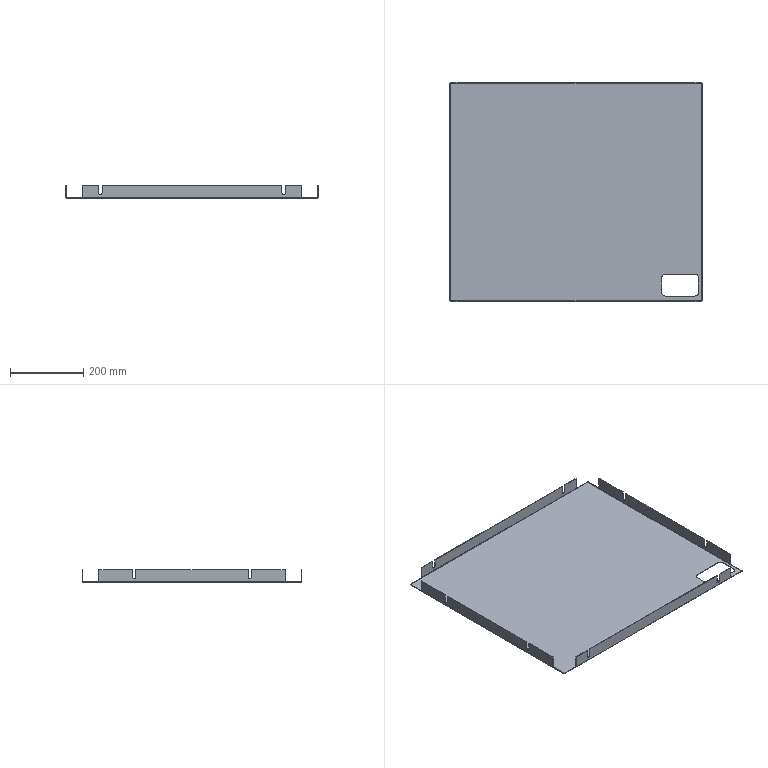Part | SolidWorks | features BaseBody 1 | 1 solid | 98 faces | box 688 x 598 x 35 mm | volume 714529 mm3 | plane 66 | cylinder 24 | spline 8 | commonest cylinder face diameters 9 x12 1.473 x4 4.473 x4 20 x4